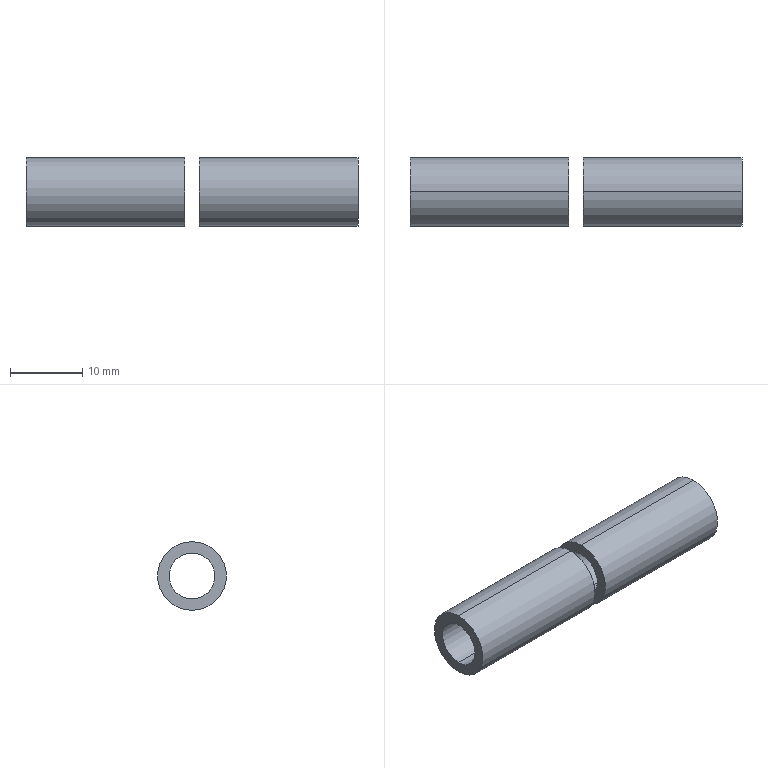Part | SolidWorks | features BaseBody 2 | 2 solids | 12 faces | box 46 x 9.5 x 9.5 mm | volume 1724 mm3 | cylinder 8 | plane 4 | commonest cylinder face diameters 6.35 x4 9.5 x4
STEP:
#1=CARTESIAN_POINT('',(-23.,-89.989,-985.163));
#2=VERTEX_POINT('',#1);
#3=CARTESIAN_POINT('',(-23.,-89.989,-978.813));
#4=VERTEX_POINT('',#3);
#5=CARTESIAN_POINT('',(-23.,-89.989,-981.988));
#6=DIRECTION('',(-1.,0.,0.));
#7=DIRECTION('',(0.,0.,-1.));
#8=AXIS2_PLACEMENT_3D('',#5,#6,#7);
#9=CIRCLE('',#8,3.175);
#10=EDGE_CURVE('',#2,#4,#9,.T.);
#11=ORIENTED_EDGE('',*,*,#10,.T.);
#12=CARTESIAN_POINT('',(-1.016,-89.989,-978.813));
#13=VERTEX_POINT('',#12);
#14=CARTESIAN_POINT('',(-23.,-89.989,-978.813));
#15=DIRECTION('',(1.,0.,0.));
#16=VECTOR('',#15,1000.);
#17=LINE('',#14,#16);
#18=EDGE_CURVE('',#4,#13,#17,.T.);
#19=ORIENTED_EDGE('',*,*,#18,.T.);
#20=CARTESIAN_POINT('',(-1.016,-89.989,-985.163));
#21=VERTEX_POINT('',#20);
#22=CARTESIAN_POINT('',(-1.016,-89.989,-981.988));
#23=DIRECTION('',(1.,0.,0.));
#24=DIRECTION('',(0.,0.,-1.));
#25=AXIS2_PLACEMENT_3D('',#22,#23,#24);
#26=CIRCLE('',#25,3.175);
#27=EDGE_CURVE('',#13,#21,#26,.T.);
#28=ORIENTED_EDGE('',*,*,#27,.T.);
#29=CARTESIAN_POINT('',(-23.,-89.989,-985.163));
#30=DIRECTION('',(1.,0.,0.));
#31=VECTOR('',#30,1000.);
#32=LINE('',#29,#31);
#33=EDGE_CURVE('',#2,#21,#32,.T.);
#34=ORIENTED_EDGE('',*,*,#33,.F.);
#35=EDGE_LOOP('',(#11,#19,#28,#34));
#36=FACE_OUTER_BOUND('',#35,.T.);
#37=CARTESIAN_POINT('',(-23.,-89.989,-981.988));
#38=DIRECTION('',(1.,0.,0.));
#39=DIRECTION('',(0.,0.,-1.));
#40=AXIS2_PLACEMENT_3D('',#37,#38,#39);
#41=CYLINDRICAL_SURFACE('',#40,3.175);
#42=ADVANCED_FACE('',(#36),#41,.F.);
#43=CARTESIAN_POINT('',(-23.,-89.989,-986.738));
#44=VERTEX_POINT('',#43);
#45=CARTESIAN_POINT('',(-23.,-89.989,-977.238));
#46=VERTEX_POINT('',#45);
#47=CARTESIAN_POINT('',(-23.,-89.989,-981.988));
#48=DIRECTION('',(1.,0.,0.));
#49=DIRECTION('',(0.,0.,-1.));
#50=AXIS2_PLACEMENT_3D('',#47,#48,#49);
#51=CIRCLE('',#50,4.75);
#52=EDGE_CURVE('',#44,#46,#51,.T.);
#53=ORIENTED_EDGE('',*,*,#52,.T.);
#54=CARTESIAN_POINT('',(-1.016,-89.989,-977.238));
#55=VERTEX_POINT('',#54);
#56=CARTESIAN_POINT('',(-23.,-89.989,-977.238));
#57=DIRECTION('',(1.,0.,0.));
#58=VECTOR('',#57,1000.);
#59=LINE('',#56,#58);
#60=EDGE_CURVE('',#46,#55,#59,.T.);
#61=ORIENTED_EDGE('',*,*,#60,.T.);
#62=CARTESIAN_POINT('',(-1.016,-89.989,-986.738));
#63=VERTEX_POINT('',#62);
#64=CARTESIAN_POINT('',(-1.016,-89.989,-981.988));
#65=DIRECTION('',(-1.,0.,0.));
#66=DIRECTION('',(0.,0.,-1.));
#67=AXIS2_PLACEMENT_3D('',#64,#65,#66);
#68=CIRCLE('',#67,4.75);
#69=EDGE_CURVE('',#55,#63,#68,.T.);
#70=ORIENTED_EDGE('',*,*,#69,.T.);
#71=CARTESIAN_POINT('',(-23.,-89.989,-986.738));
#72=DIRECTION('',(1.,0.,0.));
#73=VECTOR('',#72,1000.);
#74=LINE('',#71,#73);
#75=EDGE_CURVE('',#44,#63,#74,.T.);
#76=ORIENTED_EDGE('',*,*,#75,.F.);
#77=EDGE_LOOP('',(#53,#61,#70,#76));
#78=FACE_OUTER_BOUND('',#77,.T.);
#79=CARTESIAN_POINT('',(-23.,-89.989,-981.988));
#80=DIRECTION('',(1.,0.,0.));
#81=DIRECTION('',(0.,0.,-1.));
#82=AXIS2_PLACEMENT_3D('',#79,#80,#81);
#83=CYLINDRICAL_SURFACE('',#82,4.75);
#84=ADVANCED_FACE('',(#78),#83,.T.);
#85=ORIENTED_EDGE('',*,*,#18,.F.);
#86=CARTESIAN_POINT('',(-23.,-89.989,-981.988));
#87=DIRECTION('',(-1.,0.,0.));
#88=DIRECTION('',(0.,0.,-1.));
#89=AXIS2_PLACEMENT_3D('',#86,#87,#88);
#90=CIRCLE('',#89,3.175);
#91=EDGE_CURVE('',#4,#2,#90,.T.);
#92=ORIENTED_EDGE('',*,*,#91,.T.);
#93=ORIENTED_EDGE('',*,*,#33,.T.);
#94=CARTESIAN_POINT('',(-1.016,-89.989,-981.988));
#95=DIRECTION('',(1.,0.,0.));
#96=DIRECTION('',(0.,0.,-1.));
#97=AXIS2_PLACEMENT_3D('',#94,#95,#96);
#98=CIRCLE('',#97,3.175);
#99=EDGE_CURVE('',#21,#13,#98,.T.);
#100=ORIENTED_EDGE('',*,*,#99,.T.);
#101=EDGE_LOOP('',(#85,#92,#93,#100));
#102=FACE_OUTER_BOUND('',#101,.T.);
#103=CARTESIAN_POINT('',(-23.,-89.989,-981.988));
#104=DIRECTION('',(1.,0.,0.));
#105=DIRECTION('',(0.,0.,-1.));
#106=AXIS2_PLACEMENT_3D('',#103,#104,#105);
#107=CYLINDRICAL_SURFACE('',#106,3.175);
#108=ADVANCED_FACE('',(#102),#107,.F.);
#109=ORIENTED_EDGE('',*,*,#99,.F.);
#110=ORIENTED_EDGE('',*,*,#27,.F.);
#111=EDGE_LOOP('',(#109,#110));
#112=FACE_BOUND('',#111,.T.);
#113=CARTESIAN_POINT('',(-1.016,-89.989,-981.988));
#114=DIRECTION('',(-1.,0.,0.));
#115=DIRECTION('',(0.,0.,-1.));
#116=AXIS2_PLACEMENT_3D('',#113,#114,#115);
#117=CIRCLE('',#116,4.75);
#118=EDGE_CURVE('',#63,#55,#117,.T.);
#119=ORIENTED_EDGE('',*,*,#118,.F.);
#120=ORIENTED_EDGE('',*,*,#69,.F.);
#121=EDGE_LOOP('',(#119,#120));
#122=FACE_OUTER_BOUND('',#121,.T.);
#123=CARTESIAN_POINT('',(-1.016,-94.796,-986.795));
#124=DIRECTION('',(-1.,0.,0.));
#125=DIRECTION('',(0.,0.,1.));
#126=AXIS2_PLACEMENT_3D('',#123,#124,#125);
#127=PLANE('',#126);
#128=ADVANCED_FACE('',(#112,#122),#127,.F.);
#129=ORIENTED_EDGE('',*,*,#10,.F.);
#130=ORIENTED_EDGE('',*,*,#91,.F.);
#131=EDGE_LOOP('',(#129,#130));
#132=FACE_BOUND('',#131,.T.);
#133=ORIENTED_EDGE('',*,*,#52,.F.);
#134=CARTESIAN_POINT('',(-23.,-89.989,-981.988));
#135=DIRECTION('',(1.,0.,0.));
#136=DIRECTION('',(0.,0.,-1.));
#137=AXIS2_PLACEMENT_3D('',#134,#135,#136);
#138=CIRCLE('',#137,4.75);
#139=EDGE_CURVE('',#46,#44,#138,.T.);
#140=ORIENTED_EDGE('',*,*,#139,.F.);
#141=EDGE_LOOP('',(#133,#140));
#142=FACE_OUTER_BOUND('',#141,.T.);
#143=CARTESIAN_POINT('',(-23.,-85.182,-986.795));
#144=DIRECTION('',(1.,0.,0.));
#145=DIRECTION('',(0.,0.,1.));
#146=AXIS2_PLACEMENT_3D('',#143,#144,#145);
#147=PLANE('',#146);
#148=ADVANCED_FACE('',(#132,#142),#147,.F.);
#149=ORIENTED_EDGE('',*,*,#60,.F.);
#150=ORIENTED_EDGE('',*,*,#139,.T.);
#151=ORIENTED_EDGE('',*,*,#75,.T.);
#152=ORIENTED_EDGE('',*,*,#118,.T.);
#153=EDGE_LOOP('',(#149,#150,#151,#152));
#154=FACE_OUTER_BOUND('',#153,.T.);
#155=CARTESIAN_POINT('',(-23.,-89.989,-981.988));
#156=DIRECTION('',(1.,0.,0.));
#157=DIRECTION('',(0.,0.,-1.));
#158=AXIS2_PLACEMENT_3D('',#155,#156,#157);
#159=CYLINDRICAL_SURFACE('',#158,4.75);
#160=ADVANCED_FACE('',(#154),#159,.T.);
#161=CLOSED_SHELL('',(#42,#84,#108,#128,#148,#160));
#162=MANIFOLD_SOLID_BREP('',#161);
#163=CARTESIAN_POINT('',(23.,-89.989,-978.813));
#164=VERTEX_POINT('',#163);
#165=CARTESIAN_POINT('',(23.,-89.989,-985.163));
#166=VERTEX_POINT('',#165);
#167=CARTESIAN_POINT('',(23.,-89.989,-981.988));
#168=DIRECTION('',(1.,0.,0.));
#169=DIRECTION('',(0.,0.,1.));
#170=AXIS2_PLACEMENT_3D('',#167,#168,#169);
#171=CIRCLE('',#170,3.175);
#172=EDGE_CURVE('',#164,#166,#171,.T.);
#173=ORIENTED_EDGE('',*,*,#172,.T.);
#174=CARTESIAN_POINT('',(1.016,-89.989,-985.163));
#175=VERTEX_POINT('',#174);
#176=CARTESIAN_POINT('',(23.,-89.989,-985.163));
#177=DIRECTION('',(-1.,0.,0.));
#178=VECTOR('',#177,1000.);
#179=LINE('',#176,#178);
#180=EDGE_CURVE('',#166,#175,#179,.T.);
#181=ORIENTED_EDGE('',*,*,#180,.T.);
#182=CARTESIAN_POINT('',(1.016,-89.989,-978.813));
#183=VERTEX_POINT('',#182);
#184=CARTESIAN_POINT('',(1.016,-89.989,-981.988));
#185=DIRECTION('',(-1.,0.,0.));
#186=DIRECTION('',(0.,0.,1.));
#187=AXIS2_PLACEMENT_3D('',#184,#185,#186);
#188=CIRCLE('',#187,3.175);
#189=EDGE_CURVE('',#175,#183,#188,.T.);
#190=ORIENTED_EDGE('',*,*,#189,.T.);
#191=CARTESIAN_POINT('',(23.,-89.989,-978.813));
#192=DIRECTION('',(-1.,0.,0.));
#193=VECTOR('',#192,1000.);
#194=LINE('',#191,#193);
#195=EDGE_CURVE('',#164,#183,#194,.T.);
#196=ORIENTED_EDGE('',*,*,#195,.F.);
#197=EDGE_LOOP('',(#173,#181,#190,#196));
#198=FACE_OUTER_BOUND('',#197,.T.);
#199=CARTESIAN_POINT('',(23.,-89.989,-981.988));
#200=DIRECTION('',(-1.,0.,0.));
#201=DIRECTION('',(0.,0.,1.));
#202=AXIS2_PLACEMENT_3D('',#199,#200,#201);
#203=CYLINDRICAL_SURFACE('',#202,3.175);
#204=ADVANCED_FACE('',(#198),#203,.F.);
#205=CARTESIAN_POINT('',(23.,-89.989,-977.238));
#206=VERTEX_POINT('',#205);
#207=CARTESIAN_POINT('',(23.,-89.989,-986.738));
#208=VERTEX_POINT('',#207);
#209=CARTESIAN_POINT('',(23.,-89.989,-981.988));
#210=DIRECTION('',(-1.,0.,0.));
#211=DIRECTION('',(0.,0.,1.));
#212=AXIS2_PLACEMENT_3D('',#209,#210,#211);
#213=CIRCLE('',#212,4.75);
#214=EDGE_CURVE('',#206,#208,#213,.T.);
#215=ORIENTED_EDGE('',*,*,#214,.T.);
#216=CARTESIAN_POINT('',(1.016,-89.989,-986.738));
#217=VERTEX_POINT('',#216);
#218=CARTESIAN_POINT('',(23.,-89.989,-986.738));
#219=DIRECTION('',(-1.,0.,0.));
#220=VECTOR('',#219,1000.);
#221=LINE('',#218,#220);
#222=EDGE_CURVE('',#208,#217,#221,.T.);
#223=ORIENTED_EDGE('',*,*,#222,.T.);
#224=CARTESIAN_POINT('',(1.016,-89.989,-977.238));
#225=VERTEX_POINT('',#224);
#226=CARTESIAN_POINT('',(1.016,-89.989,-981.988));
#227=DIRECTION('',(1.,0.,0.));
#228=DIRECTION('',(0.,0.,1.));
#229=AXIS2_PLACEMENT_3D('',#226,#227,#228);
#230=CIRCLE('',#229,4.75);
#231=EDGE_CURVE('',#217,#225,#230,.T.);
#232=ORIENTED_EDGE('',*,*,#231,.T.);
#233=CARTESIAN_POINT('',(23.,-89.989,-977.238));
#234=DIRECTION('',(-1.,0.,0.));
#235=VECTOR('',#234,1000.);
#236=LINE('',#233,#235);
#237=EDGE_CURVE('',#206,#225,#236,.T.);
#238=ORIENTED_EDGE('',*,*,#237,.F.);
#239=EDGE_LOOP('',(#215,#223,#232,#238));
#240=FACE_OUTER_BOUND('',#239,.T.);
#241=CARTESIAN_POINT('',(23.,-89.989,-981.988));
#242=DIRECTION('',(-1.,0.,0.));
#243=DIRECTION('',(0.,0.,1.));
#244=AXIS2_PLACEMENT_3D('',#241,#242,#243);
#245=CYLINDRICAL_SURFACE('',#244,4.75);
#246=ADVANCED_FACE('',(#240),#245,.T.);
#247=ORIENTED_EDGE('',*,*,#180,.F.);
#248=CARTESIAN_POINT('',(23.,-89.989,-981.988));
#249=DIRECTION('',(1.,0.,0.));
#250=DIRECTION('',(0.,0.,1.));
#251=AXIS2_PLACEMENT_3D('',#248,#249,#250);
#252=CIRCLE('',#251,3.175);
#253=EDGE_CURVE('',#166,#164,#252,.T.);
#254=ORIENTED_EDGE('',*,*,#253,.T.);
#255=ORIENTED_EDGE('',*,*,#195,.T.);
#256=CARTESIAN_POINT('',(1.016,-89.989,-981.988));
#257=DIRECTION('',(-1.,0.,0.));
#258=DIRECTION('',(0.,0.,1.));
#259=AXIS2_PLACEMENT_3D('',#256,#257,#258);
#260=CIRCLE('',#259,3.175);
#261=EDGE_CURVE('',#183,#175,#260,.T.);
#262=ORIENTED_EDGE('',*,*,#261,.T.);
#263=EDGE_LOOP('',(#247,#254,#255,#262));
#264=FACE_OUTER_BOUND('',#263,.T.);
#265=CARTESIAN_POINT('',(23.,-89.989,-981.988));
#266=DIRECTION('',(-1.,0.,0.));
#267=DIRECTION('',(0.,0.,1.));
#268=AXIS2_PLACEMENT_3D('',#265,#266,#267);
#269=CYLINDRICAL_SURFACE('',#268,3.175);
#270=ADVANCED_FACE('',(#264),#269,.F.);
#271=ORIENTED_EDGE('',*,*,#261,.F.);
#272=ORIENTED_EDGE('',*,*,#189,.F.);
#273=EDGE_LOOP('',(#271,#272));
#274=FACE_BOUND('',#273,.T.);
#275=CARTESIAN_POINT('',(1.016,-89.989,-981.988));
#276=DIRECTION('',(1.,0.,0.));
#277=DIRECTION('',(0.,0.,1.));
#278=AXIS2_PLACEMENT_3D('',#275,#276,#277);
#279=CIRCLE('',#278,4.75);
#280=EDGE_CURVE('',#225,#217,#279,.T.);
#281=ORIENTED_EDGE('',*,*,#280,.F.);
#282=ORIENTED_EDGE('',*,*,#231,.F.);
#283=EDGE_LOOP('',(#281,#282));
#284=FACE_OUTER_BOUND('',#283,.T.);
#285=CARTESIAN_POINT('',(1.016,-94.796,-977.181));
#286=DIRECTION('',(1.,0.,0.));
#287=DIRECTION('',(0.,0.,-1.));
#288=AXIS2_PLACEMENT_3D('',#285,#286,#287);
#289=PLANE('',#288);
#290=ADVANCED_FACE('',(#274,#284),#289,.F.);
#291=ORIENTED_EDGE('',*,*,#172,.F.);
#292=ORIENTED_EDGE('',*,*,#253,.F.);
#293=EDGE_LOOP('',(#291,#292));
#294=FACE_BOUND('',#293,.T.);
#295=ORIENTED_EDGE('',*,*,#214,.F.);
#296=CARTESIAN_POINT('',(23.,-89.989,-981.988));
#297=DIRECTION('',(-1.,0.,0.));
#298=DIRECTION('',(0.,0.,1.));
#299=AXIS2_PLACEMENT_3D('',#296,#297,#298);
#300=CIRCLE('',#299,4.75);
#301=EDGE_CURVE('',#208,#206,#300,.T.);
#302=ORIENTED_EDGE('',*,*,#301,.F.);
#303=EDGE_LOOP('',(#295,#302));
#304=FACE_OUTER_BOUND('',#303,.T.);
#305=CARTESIAN_POINT('',(23.,-94.796,-986.795));
#306=DIRECTION('',(-1.,0.,0.));
#307=DIRECTION('',(0.,0.,1.));
#308=AXIS2_PLACEMENT_3D('',#305,#306,#307);
#309=PLANE('',#308);
#310=ADVANCED_FACE('',(#294,#304),#309,.F.);
#311=ORIENTED_EDGE('',*,*,#222,.F.);
#312=ORIENTED_EDGE('',*,*,#301,.T.);
#313=ORIENTED_EDGE('',*,*,#237,.T.);
#314=ORIENTED_EDGE('',*,*,#280,.T.);
#315=EDGE_LOOP('',(#311,#312,#313,#314));
#316=FACE_OUTER_BOUND('',#315,.T.);
#317=CARTESIAN_POINT('',(23.,-89.989,-981.988));
#318=DIRECTION('',(-1.,0.,0.));
#319=DIRECTION('',(0.,0.,1.));
#320=AXIS2_PLACEMENT_3D('',#317,#318,#319);
#321=CYLINDRICAL_SURFACE('',#320,4.75);
#322=ADVANCED_FACE('',(#316),#321,.T.);
#323=CLOSED_SHELL('',(#204,#246,#270,#290,#310,#322));
#324=MANIFOLD_SOLID_BREP('',#323);
#325=CARTESIAN_POINT('',(0.,0.,0.));
#326=DIRECTION('',(0.,0.,1.));
#327=DIRECTION('',(1.,0.,0.));
#328=AXIS2_PLACEMENT_3D('',#325,#326,#327);
#329=(LENGTH_UNIT()NAMED_UNIT(*)SI_UNIT(.MILLI.,.METRE.));
#330=UNCERTAINTY_MEASURE_WITH_UNIT(LENGTH_MEASURE(0.00001),#329,'','');
#331=(NAMED_UNIT(*)PLANE_ANGLE_UNIT()SI_UNIT($,.RADIAN.));
#332=(NAMED_UNIT(*)SI_UNIT($,.STERADIAN.)SOLID_ANGLE_UNIT());
#333=(GEOMETRIC_REPRESENTATION_CONTEXT(3)GLOBAL_UNCERTAINTY_ASSIGNED_CONTEXT((#330))GLOBAL_UNIT_ASSIGNED_CONTEXT((#329,#331,#332))REPRESENTATION_CONTEXT('',''));
#334=ADVANCED_BREP_SHAPE_REPRESENTATION('',(#162,#324,#328),#333);